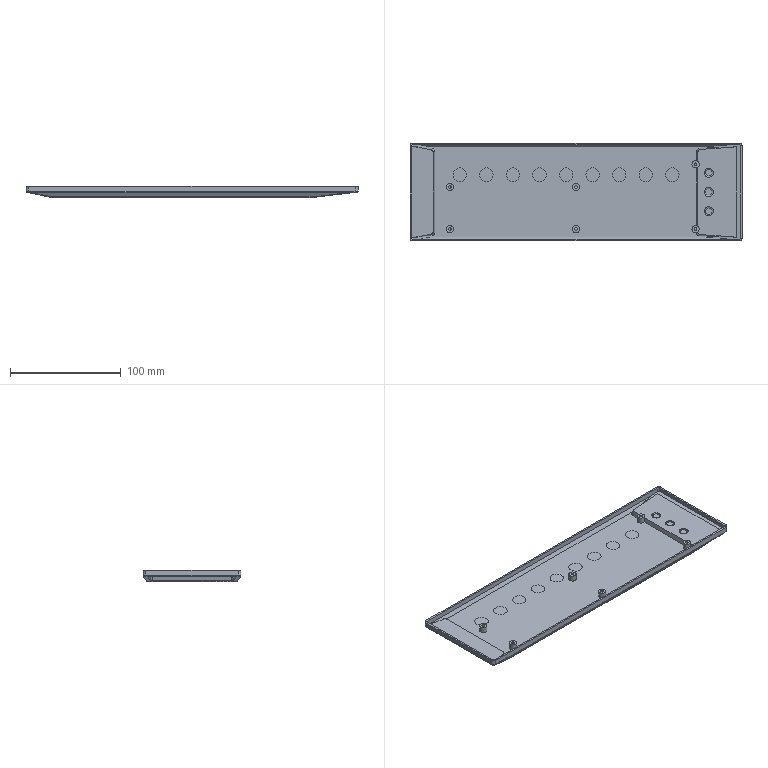NC program | NX | posted with a generic post | part box 300 x 88.5 x 10 mm
Lines 12015 to 12910 of 32249:
(CAVITY_MILL_COPY_COPY , TOOL : D2)
N23998 T02 M6
N24000 G54
N24002 G17 G0 G90 X-145.55 Y41.35 S9500 M3
N24004 G43 Z30. H2
N24006 Z0.808
N24008 G94 G1 Z-0.192 F1000.
N24010 X-145.586 Y41.393
N24012 G3 X-146.352 Y41.75 R1.
N24014 G1 X-147.5 F1100.
N24016 Y40.602
N24018 G3 X-147.143 Y39.836 R1.
N24020 G1 X-147.1 Y39.8
N24022 Z0.808
N24024 G0 Z30.
N24026 X-145.55 Y41.35
N24028 Z0.615
N24030 G1 Z-0.385 F1000.
N24032 X-145.586 Y41.393
N24034 G3 X-146.352 Y41.75 R1.
N24036 G1 X-147.5 F1100.
N24038 Y40.602
N24040 G3 X-147.143 Y39.836 R1.
N24042 G1 X-147.1 Y39.8
N24044 Z0.615
N24046 G0 Z30.
N24048 X-145.55 Y41.35
N24050 Z0.423
N24052 G1 Z-0.577 F1000.
N24054 X-145.586 Y41.393
N24056 G3 X-146.352 Y41.75 R1.
N24058 G1 X-147.5 F1100.
N24060 Y40.602
N24062 G3 X-147.143 Y39.836 R1.
N24064 G1 X-147.1 Y39.8
N24066 Z0.423
N24068 G0 Z30.
N24070 X-145.55 Y41.35
N24072 Z0.231
N24074 G1 Z-0.769 F1000.
N24076 X-145.586 Y41.393
N24078 G3 X-146.352 Y41.75 R1.
N24080 G1 X-147.5 F1100.
N24082 Y40.602
N24084 G3 X-147.143 Y39.836 R1.
N24086 G1 X-147.1 Y39.8
N24088 Z0.231
N24090 G0 Z30.
N24092 X-145.55 Y41.35
N24094 Z0.038
N24096 G1 Z-0.962 F1000.
N24098 X-145.586 Y41.393
N24100 G3 X-146.352 Y41.75 R1.
N24102 G1 X-147.5 F1100.
N24104 Y40.602
N24106 G3 X-147.143 Y39.836 R1.
N24108 G1 X-147.1 Y39.8
N24110 Z0.038
N24112 G0 X-145.55 Y41.35 Z-0.154
N24114 G1 Z-1.154 F1000.
N24116 X-145.586 Y41.393
N24118 G3 X-146.352 Y41.75 R1.
N24120 G1 X-147.5 F1100.
N24122 Y40.602
N24124 G3 X-147.143 Y39.836 R1.
N24126 G1 X-147.1 Y39.8
N24128 Z-0.154
N24130 G0 X-145.55 Y41.35 Z-0.346
N24132 G1 Z-1.346 F1000.
N24134 X-145.586 Y41.393
N24136 G3 X-146.352 Y41.75 R1.
N24138 G1 X-147.5 F1100.
N24140 Y40.602
N24142 G3 X-147.143 Y39.836 R1.
N24144 G1 X-147.1 Y39.8
N24146 Z-0.346
N24148 G0 X-145.55 Y41.35 Z-0.538
N24150 G1 Z-1.538 F1000.
N24152 X-145.586 Y41.393
N24154 G3 X-146.352 Y41.75 R1.
N24156 G1 X-147.5 F1100.
N24158 Y40.602
N24160 G3 X-147.143 Y39.836 R1.
N24162 G1 X-147.1 Y39.8
N24164 Z-0.538
N24166 G0 X-145.55 Y41.35 Z-0.731
N24168 G1 Z-1.731 F1000.
N24170 X-145.586 Y41.393
N24172 G3 X-146.352 Y41.75 R1.
N24174 G1 X-147.5 F1100.
N24176 Y40.602
N24178 G3 X-147.143 Y39.836 R1.
N24180 G1 X-147.1 Y39.8
N24182 Z-0.731
N24184 G0 X-145.55 Y41.35 Z-0.923
N24186 G1 Z-1.923 F1000.
N24188 X-145.586 Y41.393
N24190 G3 X-146.352 Y41.75 R1.
N24192 G1 X-147.5 F1100.
N24194 Y40.602
N24196 G3 X-147.143 Y39.836 R1.
N24198 G1 X-147.1 Y39.8
N24200 Z-0.923
N24202 G0 X-145.55 Y41.35 Z-1.115
N24204 G1 Z-2.115 F1000.
N24206 X-145.586 Y41.393
N24208 G3 X-146.352 Y41.75 R1.
N24210 G1 X-147.5 F1100.
N24212 Y40.602
N24214 G3 X-147.143 Y39.836 R1.
N24216 G1 X-147.1 Y39.8
N24218 Z-1.115
N24220 G0 X-145.55 Y41.35 Z-1.308
N24222 G1 Z-2.308 F1000.
N24224 X-145.586 Y41.393
N24226 G3 X-146.352 Y41.75 R1.
N24228 G1 X-147.5 F1100.
N24230 Y40.602
N24232 G3 X-147.143 Y39.836 R1.
N24234 G1 X-147.1 Y39.8
N24236 Z-1.308
N24238 G0 X-145.55 Y41.35 Z-1.5
N24240 G1 Z-2.5 F1000.
N24242 X-145.586 Y41.393
N24244 G3 X-146.352 Y41.75 R1.
N24246 G1 X-147.5 F1100.
N24248 Y40.602
N24250 G3 X-147.143 Y39.836 R1.
N24252 G1 X-147.1 Y39.8
N24254 Z-1.5
N24256 G0 X-145.55 Y41.35 Z-1.692
N24258 G1 Z-2.692 F1000.
N24260 X-145.586 Y41.393
N24262 G3 X-146.352 Y41.75 R1.
N24264 G1 X-147.5 F1100.
N24266 Y40.602
N24268 G3 X-147.143 Y39.836 R1.
N24270 G1 X-147.1 Y39.8
N24272 Z-1.692
N24274 G0 X-145.55 Y41.35 Z-1.883
N24276 G1 Z-2.883 F1000.
N24278 X-145.586 Y41.393
N24280 G3 X-146.352 Y41.75 R1.
N24282 G1 X-147.5 F1100.
N24284 Y40.602
N24286 G3 X-147.143 Y39.836 R1.
N24288 G1 X-147.1 Y39.8
N24290 Z-1.883
N24292 G0 X-145.55 Y41.35 Z-2.075
N24294 G1 Z-3.075 F1000.
N24296 X-145.586 Y41.393
N24298 G3 X-146.352 Y41.75 R1.
N24300 G1 X-147.5 F1100.
N24302 Y40.602
N24304 G3 X-147.143 Y39.836 R1.
N24306 G1 X-147.1 Y39.8
N24308 Z-2.075
N24310 G0 X-145.55 Y41.35 Z-2.267
N24312 G1 Z-3.267 F1000.
N24314 X-145.586 Y41.393
N24316 G3 X-146.352 Y41.75 R1.
N24318 G1 X-147.5 F1100.
N24320 Y40.602
N24322 G3 X-147.143 Y39.836 R1.
N24324 G1 X-147.1 Y39.8
N24326 Z-2.267
N24328 G0 X-145.55 Y41.35 Z-2.458
N24330 G1 Z-3.458 F1000.
N24332 X-145.586 Y41.393
N24334 G3 X-146.352 Y41.75 R1.
N24336 G1 X-147.5 F1100.
N24338 Y40.602
N24340 G3 X-147.143 Y39.836 R1.
N24342 G1 X-147.1 Y39.8
N24344 Z-2.458
N24346 G0 X-145.55 Y41.35 Z-2.65
N24348 G1 Z-3.65 F1000.
N24350 X-145.586 Y41.393
N24352 G3 X-146.352 Y41.75 R1.
N24354 G1 X-147.5 F1100.
N24356 Y40.602
N24358 G3 X-147.143 Y39.836 R1.
N24360 G1 X-147.1 Y39.8
N24362 Z-2.65
N24364 G0 X-132.444 Y41.35 Z-2.8
N24366 G1 Z-3.8 F1000.
N24368 X-132.48 Y41.393
N24370 G3 X-133.246 Y41.75 R1.
N24372 G1 X-144.825 F1100.
N24374 X-133.422 Y39.739
N24376 G3 X-132.606 Y39.958 R1.
N24378 G1 X-132.563 Y39.994
N24380 Z-2.8
N24382 G0 X-132.213 Y41.35 Z-2.95
N24384 G1 Z-3.95 F1000.
N24386 X-132.249 Y41.393
N24388 G3 X-133.015 Y41.75 R1.
N24390 G1 X-144.593 F1100.
N24392 X-133.191 Y39.739
N24394 G3 X-132.374 Y39.958 R1.
N24396 G1 X-132.331 Y39.994
N24398 Z-2.95
N24400 G0 X-131.993 Y41.35 Z-3.1
N24402 G1 Z-4.1 F1000.
N24404 X-132.029 Y41.393
N24406 G3 X-132.795 Y41.75 R1.
N24408 G1 X-144.373 F1100.
N24410 X-132.971 Y39.739
N24412 G3 X-132.154 Y39.958 R1.
N24414 G1 X-132.112 Y39.994
N24416 Z-3.1
N24418 G0 X-131.68 Y41.35 Z-3.295
N24420 G1 Z-4.295 F1000.
N24422 X-131.716 Y41.393
N24424 G3 X-132.482 Y41.75 R1.
N24426 G1 X-144.061 F1100.
N24428 X-132.658 Y39.739
N24430 G3 X-131.842 Y39.958 R1.
N24432 G1 X-131.799 Y39.994
N24434 Z-3.295
N24436 G0 X-131.38 Y41.35 Z-3.49
N24438 G1 Z-4.49 F1000.
N24440 X-131.415 Y41.393
N24442 G3 X-132.181 Y41.75 R1.
N24444 G1 X-143.76 F1100.
N24446 X-132.357 Y39.739
N24448 G3 X-131.541 Y39.958 R1.
N24450 G1 X-131.498 Y39.994
N24452 Z-3.49
N24454 G0 X-130.737 Y41.29 Z-3.685
N24456 G1 Z-4.685 F1000.
N24458 X-130.773 Y41.333
N24460 G3 X-131.539 Y41.69 R1.
N24462 G1 X-143.117 F1100.
N24464 X-131.715 Y39.679
N24466 G3 X-130.898 Y39.898 R1.
N24468 G1 X-130.855 Y39.934
N24470 Z-3.685
N24472 G0 X-129.744 Y41.173 Z-3.88
N24474 G1 Z-4.88 F1000.
N24476 X-129.78 Y41.216
N24478 G3 X-130.546 Y41.573 R1.
N24480 G1 X-142.153 F1100.
N24482 X-130.891 Y39.587
N24484 X-130.71 Y39.55
N24486 G3 X-129.907 Y39.71 R1.
N24488 G1 Z-3.88
N24490 G0 X-129.1 Y41.056 Z-4.075
N24492 G1 Z-5.075 F1000.
N24494 X-129.136 Y41.099
N24496 G3 X-129.902 Y41.456 R1.
N24498 G1 X-141.188 F1100.
N24500 X-130.839 Y39.631
N24502 G2 X-130.193 Y39.457 R3.907
N24504 G3 X-129.377 Y39.517 R1.
N24506 G1 Z-4.075
N24508 G0 X-128.576 Y40.939 Z-4.27
N24510 G1 Z-5.27 F1000.
N24512 X-128.612 Y40.982
N24514 G3 X-129.378 Y41.339 R1.
N24516 G1 X-140.224 F1100.
N24518 X-130.787 Y39.675
N24520 G2 X-129.744 Y39.334 R3.898
N24522 G3 X-128.927 Y39.305 R1.
N24524 G1 Z-4.27
N24526 G0 X-128.195 Y40.822 Z-4.465
N24528 G1 Z-5.465 F1000.
N24530 X-128.231 Y40.865
N24532 G3 X-128.997 Y41.222 R1.
N24534 G1 X-139.259 F1100.
N24536 X-130.735 Y39.719
N24538 G2 X-129.445 Y39.245 R3.898
N24540 G3 X-128.631 Y39.157 R1.
N24542 G1 Z-4.465
N24544 G0 X-127.861 Y40.705 Z-4.66
N24546 G1 Z-5.66 F1000.
N24548 X-127.897 Y40.748
N24550 G3 X-128.663 Y41.105 R1.
N24552 G1 X-138.295 F1100.
N24554 X-130.682 Y39.762
N24556 G2 X-129.177 Y39.154 R3.898
N24558 G3 X-128.372 Y39.013 R1.
N24560 G1 Z-4.66
N24562 G0 X-127.567 Y40.588 Z-4.855
N24564 G1 Z-5.855 F1000.
N24566 X-127.603 Y40.631
N24568 G3 X-128.369 Y40.988 R1.
N24570 G1 X-137.331 F1100.
N24572 X-130.63 Y39.806
N24574 G2 X-128.944 Y39.067 R3.898
N24576 G3 X-128.147 Y38.881 R1.
N24578 G1 Z-4.855
N24580 G0 X-127.285 Y40.471 Z-5.05
N24582 G1 Z-6.05 F1000.
N24584 X-127.321 Y40.514
N24586 G3 X-128.087 Y40.871 R1.
N24588 G1 X-136.366 F1100.
N24590 X-130.578 Y39.85
N24592 G2 X-128.702 Y38.953 R3.908
N24594 G3 X-127.919 Y38.716 R1.
N24596 G1 Z-5.05
N24598 G0 X-127.029 Y40.354 Z-5.245
N24600 G1 Z-6.245 F1000.
N24602 X-127.065 Y40.397
N24604 G3 X-127.831 Y40.754 R1.
N24606 G1 X-135.402 F1100.
N24608 X-130.526 Y39.894
N24610 G2 X-128.482 Y38.838 R3.919
N24612 G3 X-127.714 Y38.555 R1.
N24614 G1 Z-5.245
N24616 G0 X-126.805 Y40.237 Z-5.44
N24618 G1 Z-6.44 F1000.
N24620 X-126.841 Y40.28
N24622 G3 X-127.607 Y40.637 R1.
N24624 G1 X-134.437 F1100.
N24626 X-130.473 Y39.938
N24628 G2 X-128.3 Y38.746 R3.927
N24630 G3 X-127.547 Y38.426 R1.
N24632 G1 Z-5.44
N24634 G0 X-126.594 Y40.12 Z-5.635
N24636 G1 Z-6.635 F1000.
N24638 X-126.63 Y40.163
N24640 G3 X-127.396 Y40.52 R1.
N24642 G1 X-133.473 F1100.
N24644 X-130.421 Y39.982
N24646 G2 X-128.129 Y38.653 R3.931
N24648 G3 X-127.391 Y38.299 R1.
N24650 G1 Z-5.635
N24652 G0 X-126.395 Y40.003 Z-5.83
N24654 G1 Z-6.83 F1000.
N24656 X-126.431 Y40.046
N24658 G3 X-127.197 Y40.403 R1.
N24660 G1 X-132.508 F1100.
N24662 X-130.369 Y40.025
N24664 G2 X-127.973 Y38.578 R3.928
N24666 G3 X-127.249 Y38.196 R1.
N24668 G1 Z-5.83
N24670 G0 X-126.205 Y39.886 Z-6.025
N24672 G1 Z-7.025 F1000.
N24674 X-126.241 Y39.929
N24676 G3 X-127.007 Y40.286 R1.
N24678 G1 X-131.544 F1100.
N24680 X-130.317 Y40.069
N24682 G2 X-127.818 Y38.489 R3.9
N24684 G3 X-127.112 Y38.074 R1.
N24686 G1 Z-6.025
N24688 G0 X-126.038 Y39.769 Z-6.22
N24690 G1 Z-7.22 F1000.
N24692 X-126.074 Y39.812
N24694 G3 X-126.84 Y40.169 R1.
N24696 G1 X-130.58 F1100.
N24698 X-130.264 Y40.113
N24700 G2 X-127.686 Y38.412 R3.909
N24702 G3 X-126.996 Y37.972 R1.
N24704 G1 Z-6.22
N24706 G0 X-125.871 Y39.652 Z-6.415
N24708 G1 Z-7.415 F1000.
N24710 X-125.907 Y39.695
N24712 G3 X-126.673 Y40.052 R1.
N24714 G1 X-129.765 F1100.
N24716 G2 X-127.55 Y38.33 R3.897
N24718 G3 X-126.878 Y37.863 R1.
N24720 G1 Z-6.415
N24722 G0 X-125.709 Y39.535 Z-6.61
N24724 G1 Z-7.61 F1000.
N24726 X-125.745 Y39.578
N24728 G3 X-126.511 Y39.935 R1.
N24730 G1 X-129.268 F1100.
N24732 G2 X-127.415 Y38.229 R3.907
N24734 G3 X-126.764 Y37.733 R1.
N24736 G1 Z-6.61
N24738 G0 X-125.57 Y39.418 Z-6.805
N24740 G1 Z-7.805 F1000.
N24742 X-125.606 Y39.461
N24744 G3 X-126.372 Y39.818 R1.
N24746 G1 X-128.609 F1100.
N24748 Y39.654
N24750 G2 X-127.304 Y38.162 R3.943
N24752 G3 X-126.67 Y37.644 R1.
N24754 G1 Z-6.805
N24756 G0 X-125.497 Y39.305 Z-7.
N24758 G1 Z-8. F1000.
N24760 X-125.533 Y39.348
N24762 G3 X-126.299 Y39.705 R1.
N24764 G1 X-127.727 F1100.
N24766 Y38.981
N24768 X-127.734 Y38.947
N24770 G2 X-127.203 Y38.101 R3.964
N24772 G3 X-126.585 Y37.564 R1.
N24774 G1 Z-7.
N24776 G0 Z30.
N24778 X-147.1 Y-39.8
N24780 Z0.808
N24782 G1 Z-0.192 F1000.
N24784 X-147.143 Y-39.836
N24786 G3 X-147.5 Y-40.602 R1.
N24788 G1 Y-41.75 F1100.
N24790 X-146.352
N24792 G3 X-145.586 Y-41.393 R1.
N24794 G1 X-145.55 Y-41.35
N24796 Z0.808
N24798 G0 Z30.
N24800 X-147.1 Y-39.8
N24802 Z0.615
N24804 G1 Z-0.385 F1000.
N24806 X-147.143 Y-39.836
N24808 G3 X-147.5 Y-40.602 R1.
N24810 G1 Y-41.75 F1100.
N24812 X-146.352
N24814 G3 X-145.586 Y-41.393 R1.
N24816 G1 X-145.55 Y-41.35
N24818 Z0.615
N24820 G0 Z30.
N24822 X-147.1 Y-39.8
N24824 Z0.423
N24826 G1 Z-0.577 F1000.
N24828 X-147.143 Y-39.836
N24830 G3 X-147.5 Y-40.602 R1.
N24832 G1 Y-41.75 F1100.
N24834 X-146.352
N24836 G3 X-145.586 Y-41.393 R1.
N24838 G1 X-145.55 Y-41.35
N24840 Z0.423
N24842 G0 Z30.
N24844 X-147.1 Y-39.8
N24846 Z0.231
N24848 G1 Z-0.769 F1000.
N24850 X-147.143 Y-39.836
N24852 G3 X-147.5 Y-40.602 R1.
N24854 G1 Y-41.75 F1100.
N24856 X-146.352
N24858 G3 X-145.586 Y-41.393 R1.
N24860 G1 X-145.55 Y-41.35
N24862 Z0.231
N24864 G0 Z30.
N24866 X-147.1 Y-39.8
N24868 Z0.038
N24870 G1 Z-0.962 F1000.
N24872 X-147.143 Y-39.836
N24874 G3 X-147.5 Y-40.602 R1.
N24876 G1 Y-41.75 F1100.
N24878 X-146.352
N24880 G3 X-145.586 Y-41.393 R1.
N24882 G1 X-145.55 Y-41.35
N24884 Z0.038
N24886 G0 X-147.1 Y-39.8 Z-0.154
N24888 G1 Z-1.154 F1000.
N24890 X-147.143 Y-39.836
N24892 G3 X-147.5 Y-40.602 R1.
N24894 G1 Y-41.75 F1100.
N24896 X-146.352
N24898 G3 X-145.586 Y-41.393 R1.
N24900 G1 X-145.55 Y-41.35
N24902 Z-0.154
N24904 G0 X-147.1 Y-39.8 Z-0.346
N24906 G1 Z-1.346 F1000.
N24908 X-147.143 Y-39.836
N24910 G3 X-147.5 Y-40.602 R1.
N24912 G1 Y-41.75 F1100.
N24914 X-146.352
N24916 G3 X-145.586 Y-41.393 R1.
N24918 G1 X-145.55 Y-41.35
N24920 Z-0.346
N24922 G0 X-147.1 Y-39.8 Z-0.538
N24924 G1 Z-1.538 F1000.
N24926 X-147.143 Y-39.836
N24928 G3 X-147.5 Y-40.602 R1.
N24930 G1 Y-41.75 F1100.
N24932 X-146.352
N24934 G3 X-145.586 Y-41.393 R1.
N24936 G1 X-145.55 Y-41.35
N24938 Z-0.538
N24940 G0 X-147.1 Y-39.8 Z-0.731
N24942 G1 Z-1.731 F1000.
N24944 X-147.143 Y-39.836
N24946 G3 X-147.5 Y-40.602 R1.
N24948 G1 Y-41.75 F1100.
N24950 X-146.352
N24952 G3 X-145.586 Y-41.393 R1.
N24954 G1 X-145.55 Y-41.35
N24956 Z-0.731
N24958 G0 X-147.1 Y-39.8 Z-0.923
N24960 G1 Z-1.923 F1000.
N24962 X-147.143 Y-39.836
N24964 G3 X-147.5 Y-40.602 R1.
N24966 G1 X-147.499 Y-41.75 F1100.
N24968 X-146.352
N24970 G3 X-145.586 Y-41.393 R1.
N24972 G1 X-145.55 Y-41.35
N24974 Z-0.923
N24976 G0 X-147.1 Y-39.8 Z-1.115
N24978 G1 Z-2.115 F1000.
N24980 X-147.143 Y-39.836
N24982 G3 X-147.5 Y-40.602 R1.
N24984 G1 X-147.499 Y-41.75 F1100.
N24986 X-146.352
N24988 G3 X-145.586 Y-41.393 R1.
N24990 G1 X-145.55 Y-41.35
N24992 Z-1.115
N24994 G0 X-147.1 Y-39.8 Z-1.308
N24996 G1 Z-2.308 F1000.
N24998 X-147.143 Y-39.836
N25000 G3 X-147.5 Y-40.602 R1.
N25002 G1 X-147.499 Y-41.75 F1100.
N25004 X-146.352
N25006 G3 X-145.586 Y-41.393 R1.
N25008 G1 X-145.55 Y-41.35
N25010 Z-1.308
N25012 G0 X-147.1 Y-39.8 Z-1.5
N25014 G1 Z-2.5 F1000.
N25016 X-147.143 Y-39.836
N25018 G3 X-147.5 Y-40.602 R1.
N25020 G1 X-147.499 Y-41.75 F1100.
N25022 X-146.352
N25024 G3 X-145.586 Y-41.393 R1.
N25026 G1 X-145.55 Y-41.35
N25028 Z-1.5
N25030 G0 X-147.1 Y-39.8 Z-1.692
N25032 G1 Z-2.692 F1000.
N25034 X-147.143 Y-39.836
N25036 G3 X-147.5 Y-40.602 R1.
N25038 G1 X-147.499 Y-41.75 F1100.
N25040 X-146.352
N25042 G3 X-145.586 Y-41.393 R1.
N25044 G1 X-145.55 Y-41.35
N25046 Z-1.692
N25048 G0 X-147.1 Y-39.8 Z-1.883
N25050 G1 Z-2.883 F1000.
N25052 X-147.143 Y-39.836
N25054 G3 X-147.5 Y-40.602 R1.
N25056 G1 X-147.499 Y-41.75 F1100.
N25058 X-146.352
N25060 G3 X-145.586 Y-41.393 R1.
N25062 G1 X-145.55 Y-41.35
N25064 Z-1.883
N25066 G0 X-147.1 Y-39.8 Z-2.075
N25068 G1 Z-3.075 F1000.
N25070 X-147.143 Y-39.836
N25072 G3 X-147.5 Y-40.602 R1.
N25074 G1 X-147.499 Y-41.75 F1100.
N25076 X-146.352
N25078 G3 X-145.586 Y-41.393 R1.
N25080 G1 X-145.55 Y-41.35
N25082 Z-2.075
N25084 G0 X-147.1 Y-39.8 Z-2.267
N25086 G1 Z-3.267 F1000.
N25088 X-147.143 Y-39.836
N25090 G3 X-147.5 Y-40.602 R1.
N25092 G1 X-147.499 Y-41.75 F1100.
N25094 X-146.352
N25096 G3 X-145.586 Y-41.393 R1.
N25098 G1 X-145.55 Y-41.35
N25100 Z-2.267
N25102 G0 X-147.1 Y-39.8 Z-2.458
N25104 G1 Z-3.458 F1000.
N25106 X-147.143 Y-39.836
N25108 G3 X-147.5 Y-40.602 R1.
N25110 G1 X-147.499 Y-41.75 F1100.
N25112 X-146.352
N25114 G3 X-145.586 Y-41.393 R1.
N25116 G1 X-145.55 Y-41.35
N25118 Z-2.458
N25120 G0 X-147.1 Y-39.8 Z-2.65
N25122 G1 Z-3.65 F1000.
N25124 X-147.143 Y-39.836
N25126 G3 X-147.5 Y-40.602 R1.
N25128 G1 X-147.499 Y-41.75 F1100.
N25130 X-146.352
N25132 G3 X-145.586 Y-41.393 R1.
N25134 G1 X-145.55 Y-41.35
N25136 Z-2.65
N25138 G0 X-132.563 Y-39.994 Z-2.8
N25140 G1 Z-3.8 F1000.
N25142 X-132.606 Y-39.958
N25144 G3 X-133.422 Y-39.739 R1.
N25146 G1 X-144.825 Y-41.75 F1100.
N25148 X-133.246
N25150 G3 X-132.48 Y-41.393 R1.
N25152 G1 X-132.444 Y-41.35
N25154 Z-2.8
N25156 G0 X-132.331 Y-39.994 Z-2.95
N25158 G1 Z-3.95 F1000.
N25160 X-132.374 Y-39.958
N25162 G3 X-133.191 Y-39.739 R1.
N25164 G1 X-144.593 Y-41.75 F1100.
N25166 X-133.015
N25168 G3 X-132.249 Y-41.393 R1.
N25170 G1 X-132.213 Y-41.35
N25172 Z-2.95
N25174 G0 X-132.112 Y-39.994 Z-3.1
N25176 G1 Z-4.1 F1000.
N25178 X-132.154 Y-39.958
N25180 G3 X-132.971 Y-39.739 R1.
N25182 G1 X-144.373 Y-41.75 F1100.
N25184 X-132.795
N25186 G3 X-132.029 Y-41.393 R1.
N25188 G1 X-131.993 Y-41.35
N25190 Z-3.1
N25192 G0 X-131.799 Y-39.994 Z-3.295
N25194 G1 Z-4.295 F1000.
N25196 X-131.842 Y-39.958
N25198 G3 X-132.658 Y-39.739 R1.
N25200 G1 X-144.061 Y-41.75 F1100.
N25202 X-132.482
N25204 G3 X-131.716 Y-41.393 R1.
N25206 G1 X-131.68 Y-41.35
N25208 Z-3.295
N25210 G0 X-131.498 Y-39.994 Z-3.49
N25212 G1 Z-4.49 F1000.
N25214 X-131.541 Y-39.958
N25216 G3 X-132.357 Y-39.739 R1.
N25218 G1 X-143.76 Y-41.75 F1100.
N25220 X-132.181
N25222 G3 X-131.415 Y-41.393 R1.
N25224 G1 X-131.38 Y-41.35
N25226 Z-3.49
N25228 G0 X-130.855 Y-39.934 Z-3.685
N25230 G1 Z-4.685 F1000.
N25232 X-130.898 Y-39.898
N25234 G3 X-131.715 Y-39.679 R1.
N25236 G1 X-143.117 Y-41.69 F1100.
N25238 X-131.539
N25240 G3 X-130.773 Y-41.333 R1.
N25242 G1 X-130.737 Y-41.29
N25244 Z-3.685
N25246 G0 X-129.909 Y-39.711 Z-3.88
N25248 G1 Z-4.88 F1000.
N25250 G3 X-130.712 Y-39.551 R1.
N25252 G1 X-130.891 Y-39.587 F1100.
N25254 X-142.153 Y-41.573
N25256 X-130.547
N25258 G3 X-129.781 Y-41.216 R1.
N25260 G1 X-129.745 Y-41.173
N25262 Z-3.88
N25264 G0 X-129.376 Y-39.517 Z-4.075
N25266 G1 Z-5.075 F1000.
N25268 G3 X-130.192 Y-39.457 R1.
N25270 G2 X-130.839 Y-39.631 R3.907 F1100.
N25272 G1 X-141.188 Y-41.456
N25274 X-129.902
N25276 G3 X-129.136 Y-41.099 R1.
N25278 G1 X-129.1 Y-41.056
N25280 Z-4.075
N25282 G0 X-128.953 Y-39.324 Z-4.27
N25284 G1 Z-5.27 F1000.
N25286 G3 X-129.771 Y-39.347 R1.
N25288 G2 X-130.787 Y-39.675 R3.898 F1100.
N25290 G1 X-140.224 Y-41.339
N25292 X-129.395
N25294 G3 X-128.629 Y-40.982 R1.
N25296 G1 X-128.593 Y-40.939
N25298 Z-4.27
N25300 G0 X-128.633 Y-39.159 Z-4.465
N25302 G1 Z-5.465 F1000.
N25304 G3 X-129.447 Y-39.246 R1.
N25306 G2 X-130.735 Y-39.719 R3.898 F1100.
N25308 G1 X-139.259 Y-41.222
N25310 X-128.998
N25312 G3 X-128.232 Y-40.865 R1.
N25314 G1 X-128.196 Y-40.822
N25316 Z-4.465
N25318 G0 X-128.39 Y-39.031 Z-4.66
N25320 G1 Z-5.66 F1000.
N25322 G3 X-129.196 Y-39.166 R1.
N25324 G2 X-130.682 Y-39.762 R3.898 F1100.
N25326 G1 X-138.295 Y-41.105
N25328 X-128.674
N25330 G3 X-127.908 Y-40.748 R1.
N25332 G1 X-127.872 Y-40.705
N25334 Z-4.66
N25336 G0 X-128.171 Y-38.906 Z-4.855
N25338 G1 Z-5.855 F1000.
N25340 G3 X-128.969 Y-39.086 R1.
N25342 G2 X-130.63 Y-39.806 R3.898 F1100.
N25344 G1 X-137.331 Y-40.988
N25346 X-128.385
N25348 G3 X-127.619 Y-40.631 R1.
N25350 G1 X-127.583 Y-40.588
N25352 Z-4.855
N25354 G0 X-127.923 Y-38.722 Z-5.05
N25356 G1 Z-6.05 F1000.
N25358 G3 X-128.707 Y-38.958 R1.
N25360 G2 X-130.578 Y-39.85 R3.908 F1100.
N25362 G1 X-136.366 Y-40.871
N25364 X-128.09
N25366 G3 X-127.324 Y-40.514 R1.
N25368 G1 X-127.288 Y-40.471
N25370 Z-5.05
N25372 G0 X-127.722 Y-38.566 Z-5.245
N25374 G1 Z-6.245 F1000.
N25376 G3 X-128.491 Y-38.847 R1.
N25378 G2 X-130.526 Y-39.894 R3.919 F1100.
N25380 G1 X-135.402 Y-40.754
N25382 X-127.837
N25384 G3 X-127.07 Y-40.397 R1.
N25386 G1 X-127.035 Y-40.354
N25388 Z-5.245
N25390 G0 X-127.548 Y-38.428 Z-5.44
N25392 G1 Z-6.44 F1000.
N25394 G3 X-128.302 Y-38.747 R1.
N25396 G2 X-130.473 Y-39.938 R3.927 F1100.
N25398 G1 X-134.437 Y-40.637
N25400 X-127.607
N25402 G3 X-126.841 Y-40.28 R1.
N25404 G1 X-126.806 Y-40.237
N25406 Z-5.44
N25408 G0 X-127.373 Y-38.267 Z-5.635
N25410 G1 Z-6.635 F1000.
N25412 G3 X-128.108 Y-38.628 R1.
N25414 G2 X-130.421 Y-39.982 R3.931 F1100.
N25416 G1 X-133.473 Y-40.52
N25418 X-127.384
N25420 G3 X-126.618 Y-40.163 R1.
N25422 G1 X-126.582 Y-40.12
N25424 Z-5.635
N25426 G0 X-127.232 Y-38.152 Z-5.83
N25428 G1 Z-6.83 F1000.
N25430 G3 X-127.951 Y-38.545 R1.
N25432 G2 X-129.301 Y-39.674 R3.946 F1100.
N25434 X-130.369 Y-40.025 R5.701
N25436 G1 X-132.508 Y-40.403
N25438 X-127.185
N25440 G3 X-126.419 Y-40.046 R1.
N25442 G1 X-126.383 Y-40.003
N25444 Z-5.83
N25446 G0 X-127.098 Y-38.032 Z-6.025
N25448 G1 Z-7.025 F1000.
N25450 G3 X-127.799 Y-38.455 R1.
N25452 G2 X-129.301 Y-39.745 R3.94 F1100.
N25454 X-130.317 Y-40.069 R5.876
N25456 G1 X-131.544 Y-40.286
N25458 X-126.997
N25460 G3 X-126.231 Y-39.929 R1.
N25462 G1 X-126.195 Y-39.886
N25464 Z-6.025
N25466 G0 X-126.985 Y-37.946 Z-6.22
N25468 G1 Z-7.22 F1000.
N25470 G3 X-127.672 Y-38.391 R1.
N25472 G2 X-130.264 Y-40.113 R3.909 F1100.
N25474 G1 X-130.58 Y-40.169
N25476 X-126.831
N25478 G3 X-126.065 Y-39.812 R1.
N25480 G1 X-126.029 Y-39.769
N25482 Z-6.22
N25484 G0 X-126.872 Y-37.848 Z-6.415
N25486 G1 Z-7.415 F1000.
N25488 G3 X-127.542 Y-38.318 R1.
N25490 G2 X-129.766 Y-40.052 R3.897 F1100.
N25492 G1 X-126.667
N25494 G3 X-125.901 Y-39.695 R1.
N25496 G1 X-125.865 Y-39.652
N25498 Z-6.415
N25500 G0 X-126.756 Y-37.711 Z-6.61
N25502 G1 Z-7.61 F1000.
N25504 G3 X-127.404 Y-38.21 R1.
N25506 G2 X-129.268 Y-39.935 R3.908 F1100.
N25508 G1 X-126.504
N25510 G3 X-125.738 Y-39.578 R1.
N25512 G1 X-125.702 Y-39.535
N25514 Z-6.61
N25516 G0 X-126.668 Y-37.646 Z-6.805
N25518 G1 Z-7.805 F1000.
N25520 G3 X-127.303 Y-38.162 R1.
N25522 G2 X-128.609 Y-39.642 R3.892 F1100.
N25524 G1 Y-39.818
N25526 X-126.372
N25528 G3 X-125.606 Y-39.461 R1.
N25530 G1 X-125.57 Y-39.418
N25532 Z-6.805
N25534 G0 X-126.585 Y-37.563 Z-7.
N25536 G1 Z-8. F1000.
N25538 G3 X-127.203 Y-38.101 R1.
N25540 G2 X-127.734 Y-38.948 R3.962 F1100.
N25542 G1 X-127.727 Y-38.981
N25544 Y-39.705
N25546 X-126.299
N25548 G3 X-125.533 Y-39.348 R1.
N25550 G1 X-125.497 Y-39.305
N25552 Z-7.
N25554 G0 Z30.
N25556 X110.15 Y-38.987
N25558 Z-3.295
N25560 G1 Z-4.295 F1000.
N25562 G3 X109.908 Y-38.206 R1.
N25564 G2 X109.416 Y-37.507 R3.913 F1100.
N25566 X108.602 Y-37.707 R4.25
N25568 G3 X107.907 Y-38.149 R1.
N25570 G1 Z-3.295
N25572 G0 X110.046 Y-38.994 Z-3.49
N25574 G1 Z-4.49 F1000.
N25576 G3 X109.816 Y-38.209 R1.
N25578 G2 X109.351 Y-37.53 R3.905 F1100.
N25580 X108.548 Y-37.714 R4.25
N25582 G3 X107.848 Y-38.148 R1.
N25584 G1 Z-3.49
N25586 G0 X109.968 Y-39.021 Z-3.685
N25588 G1 Z-4.685 F1000.
N25590 G3 X109.745 Y-38.234 R1.
N25592 G2 X109.286 Y-37.551 R3.897 F1100.
N25594 X108.483 Y-37.722 R4.25
N25596 G3 X107.776 Y-38.145 R1.
N25598 G1 Z-3.685
N25600 G0 X109.889 Y-39.046 Z-3.88
N25602 G1 Z-4.88 F1000.
N25604 G3 X109.672 Y-38.257 R1.
N25606 G2 X109.219 Y-37.571 R3.902 F1100.
N25608 X108.417 Y-37.729 R4.25
N25610 G3 X107.704 Y-38.141 R1.
N25612 G1 Z-3.88
N25614 G0 X109.806 Y-39.066 Z-4.075
N25616 G1 Z-5.075 F1000.
N25618 G3 X109.596 Y-38.275 R1.
N25620 G2 X109.151 Y-37.591 R3.919 F1100.
N25622 X108.352 Y-37.735 R4.25
N25624 G3 X107.632 Y-38.135 R1.
N25626 G1 Z-4.075
N25628 G0 X109.728 Y-39.091 Z-4.27
N25630 G1 Z-5.27 F1000.
N25632 G3 X109.525 Y-38.298 R1.
N25634 G2 X109.086 Y-37.609 R3.91 F1100.
N25636 X108.287 Y-37.74 R4.25
N25638 G3 X107.561 Y-38.129 R1.
N25640 G1 Z-4.27
N25642 G0 X109.647 Y-39.114 Z-4.465
N25644 G1 Z-5.465 F1000.
N25646 G3 X109.452 Y-38.319 R1.
N25648 G2 X109.02 Y-37.626 R3.901 F1100.
N25650 X108.221 Y-37.744 R4.25
N25652 G3 X107.489 Y-38.122 R1.
N25654 G1 Z-4.465
N25656 G0 X109.561 Y-39.133 Z-4.66
N25658 G1 Z-5.66 F1000.
N25660 G3 X109.376 Y-38.337 R1.
N25662 G2 X108.954 Y-37.641 R3.886 F1100.
N25664 X108.156 Y-37.747 R4.25
N25666 G3 X107.419 Y-38.114 R1.
N25668 G1 Z-4.66
N25670 G0 X109.482 Y-39.151 Z-4.855
N25672 G1 Z-5.855 F1000.
N25674 G3 X109.303 Y-38.353 R1.
N25676 G2 X108.888 Y-37.656 R3.908 F1100.
N25678 X108.092 Y-37.749 R4.25
N25680 G3 X107.349 Y-38.104 R1.
N25682 G1 Z-4.855
N25684 G0 X109.297 Y-39.556 Z-5.05
N25686 G1 Z-6.05 F1000.
N25688 X109.387 Y-39.192
N25690 G3 X109.223 Y-38.362 R1.
N25692 G2 X108.82 Y-37.67 R3.917 F1100.
N25694 X108.029 Y-37.75 R4.25
N25696 G3 X107.281 Y-38.094 R1.
N25698 G1 Z-5.05
N25700 G0 X109.177 Y-39.696 Z-5.245
N25702 G1 Z-6.245 F1000.
N25704 X109.303 Y-39.21
N25706 G3 X109.149 Y-38.378 R1.
N25708 G2 X108.753 Y-37.683 R3.914 F1100.
N25710 X107.963 Y-37.75 R4.25
N25712 G3 X107.21 Y-38.082 R1.
N25714 G1 Z-5.245
N25716 G0 X108.935 Y-39.555 Z-5.44
N25718 G1 Z-6.44 F1000.
N25720 X109.14 Y-38.806
N25722 G3 X109.068 Y-38.389 R0.5
N25724 G2 X108.685 Y-37.694 R3.9 F1100.
N25726 X107.898 Y-37.749 R4.25
N25728 G3 X107.14 Y-38.07 R1.
N25730 G1 Z-5.44
N25732 G0 X108.652 Y-38.866 Z-5.635
N25734 G1 Z-6.635 F1000.
N25736 X109.055 Y-38.82
N25738 G3 X108.99 Y-38.402 R0.5
N25740 G2 X108.617 Y-37.705 R3.879 F1100.
N25742 X107.832 Y-37.747 R4.25
N25744 G3 X107.069 Y-38.056 R1.
N25746 G1 Z-5.635
N25748 G0 X108.475 Y-38.863 Z-5.83
N25750 G1 Z-6.83 F1000.
N25752 X108.994 Y-38.621
N25754 G3 X108.917 Y-38.419 R0.5
N25756 G2 X108.551 Y-37.714 R3.871 F1100.
N25758 X107.765 Y-37.743 R4.25
N25760 G3 X106.997 Y-38.04 R1.
N25762 G1 Z-5.83
N25764 G0 X108.273 Y-38.832 Z-6.025
N25766 G1 Z-7.025 F1000.
N25768 X108.546 Y-38.125
N25770 G3 X108.839 Y-38.43 R0.5
N25772 G2 X108.482 Y-37.723 R3.867 F1100.
N25774 X107.698 Y-37.739 R4.25
N25776 G3 X106.925 Y-38.024 R1.
N25778 G1 Z-6.025
N25780 G0 Z30.
N25782 X145.55 Y-41.35